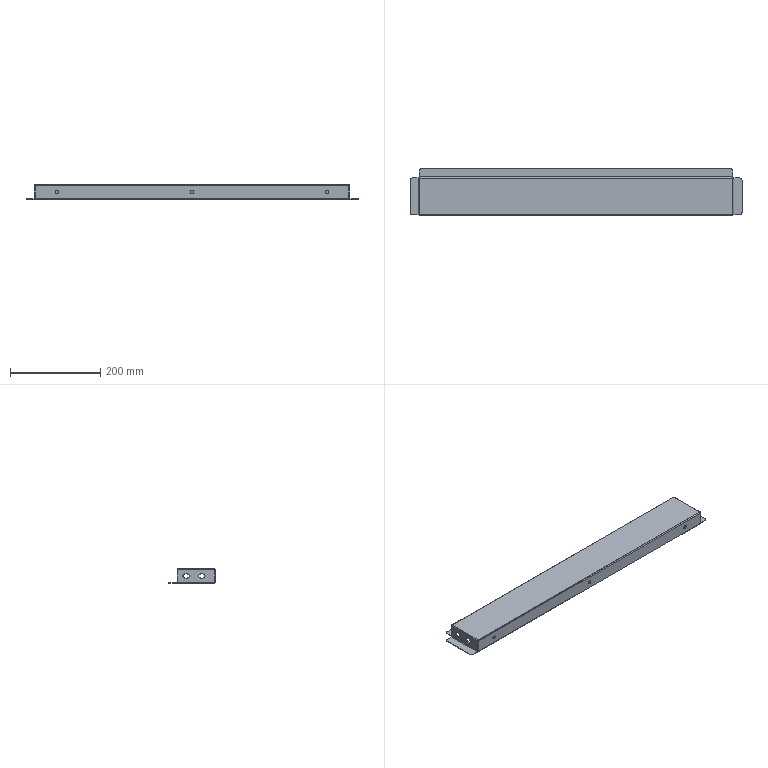Part | SolidWorks | features EdgeFlange 6, Fillet 1, FlatPattern 1, HoleWzd 1, ICE 1, SMBaseFlange 1, SheetMetal 1 | 1 solid | 98 faces | box 737.6 x 103.8 x 32 mm | volume 156480 mm3 | plane 54 | cylinder 36 | spline 8 | commonest cylinder face diameters 2 x8 4.4 x8 9 x8 7 x6 10 x6